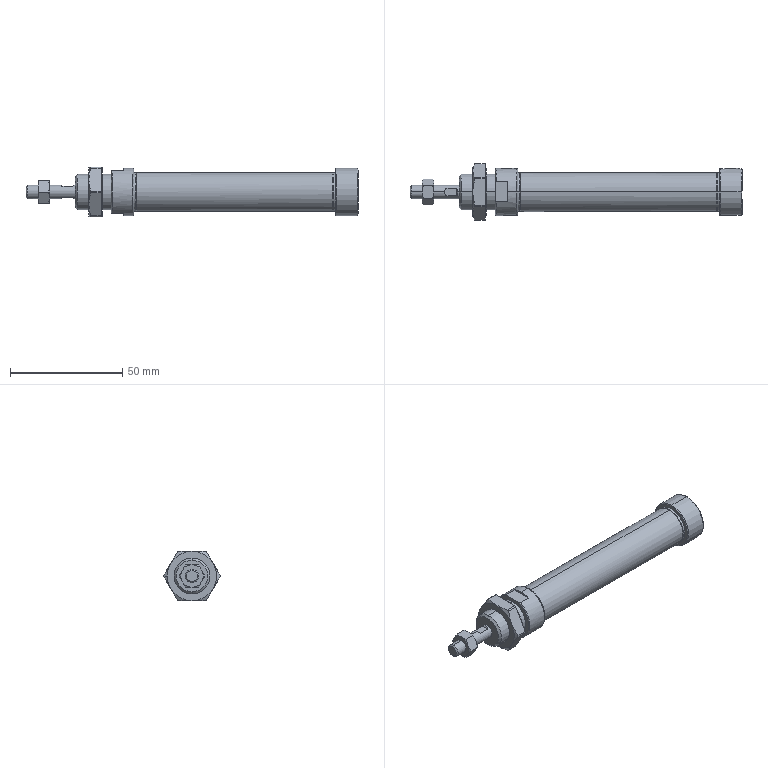Part | SolidWorks | features BaseBody 4, MoveFace 2 | 4 solids | 124 faces | box 148 x 25 x 22 mm | volume 28789 mm3 | plane 41 | cone 39 | cylinder 36 | spline 8 | commonest cylinder face diameters 17.4 x6 25 x6 4.134 x4 6 x4 16 x4 21 x4